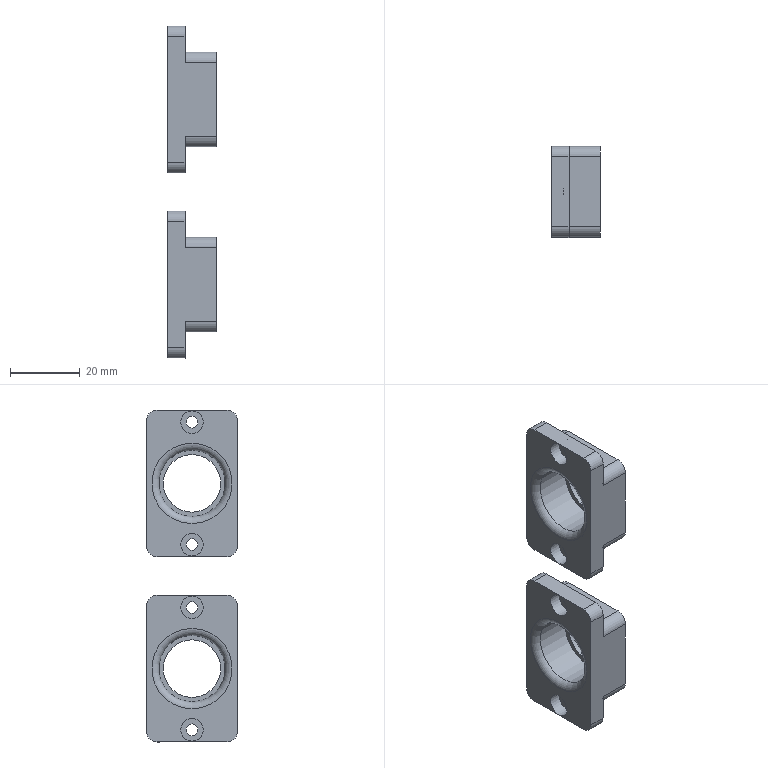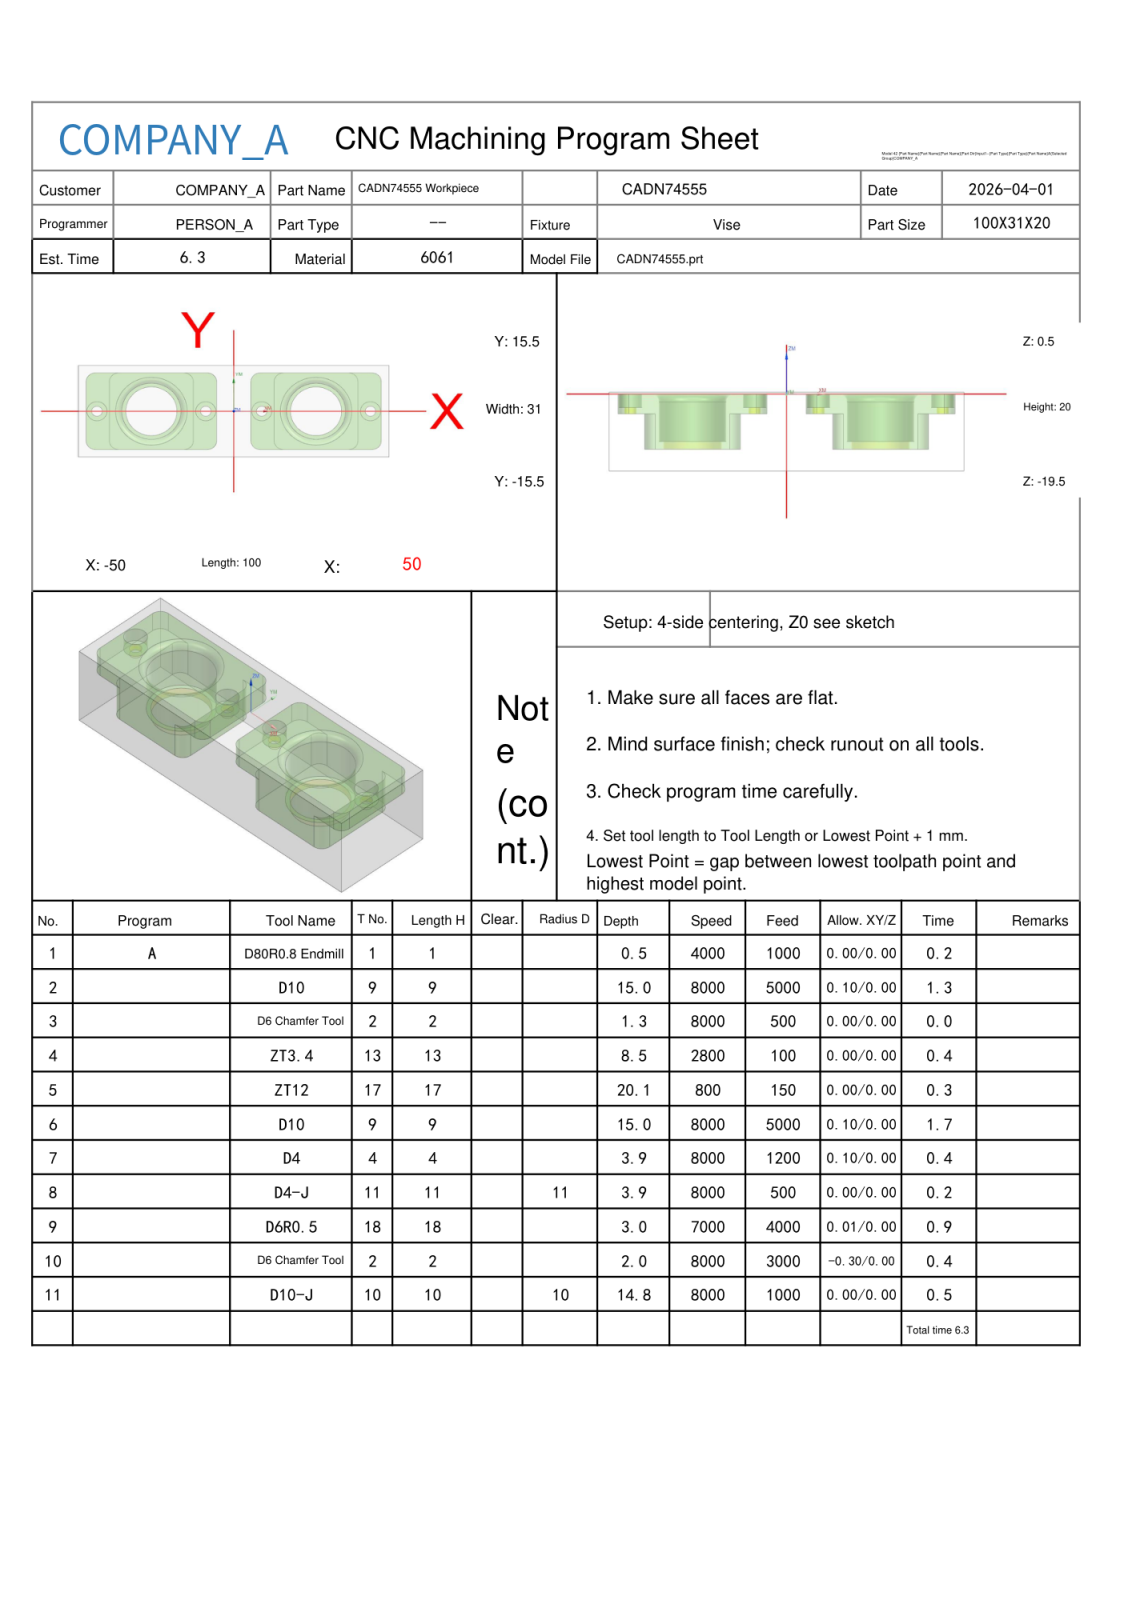NC program | NX | posted by the shop | part box 14 x 26 x 95 mm
Lines 427 to 1568 of 19918:
N6 T09 M06
(D10  D=10. R=0. H=09 ce=0.10 di=0.00)
G00 G90 G54 X-26.5 Y0.0 M03 S8000
G43 H09 Z20.
M08
Z.5
G03 X-28.7 Y-2.2 I0.0 J-2.2 F1200.
X-26.5 Y-4.4 I2.2 J0.0
X-26.5 Y-4.4 Z0.0 I0.0 J4.4
X-26.5 Y-4.4 Z-.5 I0.0 J4.4
X-26.5 Y-4.4 Z-1. I0.0 J4.4
X-26.5 Y-4.4 Z-1.5 I0.0 J4.4
X-26.5 Y-4.4 Z-2. I0.0 J4.4
X-26.5 Y-4.4 Z-2.5 I0.0 J4.4
X-26.5 Y-4.4 Z-3. I0.0 J4.4
X-26.5 Y-4.4 Z-3.5 I0.0 J4.4
X-26.5 Y-4.4 Z-4. I0.0 J4.4
X-26.5 Y-4.4 Z-4.5 I0.0 J4.4
X-26.5 Y-4.4 Z-5. I0.0 J4.4
X-26.5 Y-4.4 Z-5.5 I0.0 J4.4
X-26.5 Y-4.4 Z-6. I0.0 J4.4
X-26.5 Y-4.4 Z-6.5 I0.0 J4.4
X-26.5 Y-4.4 Z-7. I0.0 J4.4
X-26.5 Y-4.4 Z-7.5 I0.0 J4.4
X-26.5 Y-4.4 Z-8. I0.0 J4.4
X-26.5 Y-4.4 Z-8.5 I0.0 J4.4
X-26.5 Y-4.4 Z-9. I0.0 J4.4
X-26.5 Y-4.4 Z-9.5 I0.0 J4.4
X-26.5 Y-4.4 Z-10. I0.0 J4.4
X-26.5 Y-4.4 Z-10.5 I0.0 J4.4
X-26.5 Y-4.4 Z-11. I0.0 J4.4
X-26.5 Y-4.4 Z-11.5 I0.0 J4.4
X-26.5 Y-4.4 Z-12. I0.0 J4.4
X-22.1 Y0.0 I0.0 J4.4
X-26.5 Y4.4 I-4.4 J0.0
X-30.9 Y0.0 I0.0 J-4.4
X-26.5 Y-4.4 I4.4 J0.0
X-24.3 Y-2.2 I0.0 J2.2
X-26.5 Y0.0 I-2.2 J0.0
G00 Z20.
X26.5
Z.5
G03 X24.3 Y-2.2 I0.0 J-2.2
X26.5 Y-4.4 I2.2 J0.0
X26.5 Y-4.4 Z0.0 I0.0 J4.4
X26.5 Y-4.4 Z-.5 I0.0 J4.4
X26.5 Y-4.4 Z-1. I0.0 J4.4
X26.5 Y-4.4 Z-1.5 I0.0 J4.4
X26.5 Y-4.4 Z-2. I0.0 J4.4
X26.5 Y-4.4 Z-2.5 I0.0 J4.4
X26.5 Y-4.4 Z-3. I0.0 J4.4
X26.5 Y-4.4 Z-3.5 I0.0 J4.4
X26.5 Y-4.4 Z-4. I0.0 J4.4
X26.5 Y-4.4 Z-4.5 I0.0 J4.4
X26.5 Y-4.4 Z-5. I0.0 J4.4
X26.5 Y-4.4 Z-5.5 I0.0 J4.4
X26.5 Y-4.4 Z-6. I0.0 J4.4
X26.5 Y-4.4 Z-6.5 I0.0 J4.4
X26.5 Y-4.4 Z-7. I0.0 J4.4
X26.5 Y-4.4 Z-7.5 I0.0 J4.4
X26.5 Y-4.4 Z-8. I0.0 J4.4
X26.5 Y-4.4 Z-8.5 I0.0 J4.4
X26.5 Y-4.4 Z-9. I0.0 J4.4
X26.5 Y-4.4 Z-9.5 I0.0 J4.4
X26.5 Y-4.4 Z-10. I0.0 J4.4
X26.5 Y-4.4 Z-10.5 I0.0 J4.4
X26.5 Y-4.4 Z-11. I0.0 J4.4
X26.5 Y-4.4 Z-11.5 I0.0 J4.4
X26.5 Y-4.4 Z-12. I0.0 J4.4
X30.9 Y0.0 I0.0 J4.4
X26.5 Y4.4 I-4.4 J0.0
X22.1 Y0.0 I0.0 J-4.4
X26.5 Y-4.4 I4.4 J0.0
X28.7 Y-2.2 I0.0 J2.2
X26.5 Y0.0 I-2.2 J0.0
G00 Z20.
G00 G90 X-25.701 Y-3.038 M03 S8000
Z20.
Z-11.
G01 X-25.084 Y-2.847 Z-11.034 F2000.
X-24.251 Y-2.249 Z-11.088
X-23.653 Y-1.416 Z-11.141
X-23.35 Y-.436 Z-11.195
Y.436 Z-11.241
X-23.653 Y1.416 Z-11.295
X-24.251 Y2.249 Z-11.348
X-25.084 Y2.847 Z-11.402
X-26.064 Y3.15 Z-11.456
X-26.936 Z-11.501
X-27.916 Y2.847 Z-11.555
X-28.749 Y2.249 Z-11.609
X-29.347 Y1.416 Z-11.663
X-29.65 Y.436 Z-11.716
Y-.436 Z-11.762
X-29.347 Y-1.416 Z-11.816
X-28.749 Y-2.249 Z-11.87
X-27.916 Y-2.847 Z-11.923
X-26.936 Y-3.15 Z-11.977
X-26.5 Z-12.
G03 X-23.35 Y0.0 Z-12.069 I0.0 J3.15
X-26.5 Y3.15 Z-12.139 I-3.15 J0.0
X-29.65 Y0.0 Z-12.208 I0.0 J-3.15
X-26.5 Y-3.15 Z-12.278 I3.15 J0.0
X-23.35 Y0.0 Z-12.347 I0.0 J3.15
X-26.5 Y3.15 Z-12.417 I-3.15 J0.0
X-29.65 Y0.0 Z-12.486 I0.0 J-3.15
X-26.5 Y-3.15 Z-12.556 I3.15 J0.0
X-23.35 Y0.0 Z-12.625 I0.0 J3.15
X-26.5 Y3.15 Z-12.694 I-3.15 J0.0
X-29.65 Y0.0 Z-12.764 I0.0 J-3.15
X-26.5 Y-3.15 Z-12.833 I3.15 J0.0
X-23.35 Y0.0 Z-12.903 I0.0 J3.15
X-26.5 Y3.15 Z-12.972 I-3.15 J0.0
X-29.65 Y0.0 Z-13.042 I0.0 J-3.15
X-26.5 Y-3.15 Z-13.111 I3.15 J0.0
X-23.35 Y0.0 Z-13.181 I0.0 J3.15
X-26.5 Y3.15 Z-13.25 I-3.15 J0.0
X-29.65 Y0.0 Z-13.319 I0.0 J-3.15
X-26.5 Y-3.15 Z-13.389 I3.15 J0.0
X-23.35 Y0.0 Z-13.458 I0.0 J3.15
X-26.5 Y3.15 Z-13.528 I-3.15 J0.0
X-29.65 Y0.0 Z-13.597 I0.0 J-3.15
X-26.5 Y-3.15 Z-13.667 I3.15 J0.0
X-23.35 Y0.0 Z-13.736 I0.0 J3.15
X-26.5 Y3.15 Z-13.806 I-3.15 J0.0
X-29.65 Y0.0 Z-13.875 I0.0 J-3.15
X-26.5 Y-3.15 Z-13.944 I3.15 J0.0
X-23.35 Y0.0 Z-14.014 I0.0 J3.15
X-26.5 Y3.15 Z-14.083 I-3.15 J0.0
X-29.65 Y0.0 Z-14.153 I0.0 J-3.15
X-26.5 Y-3.15 Z-14.222 I3.15 J0.0
X-23.35 Y0.0 Z-14.292 I0.0 J3.15
X-26.5 Y3.15 Z-14.361 I-3.15 J0.0
X-29.65 Y0.0 Z-14.431 I0.0 J-3.15
X-26.5 Y-3.15 Z-14.5 I3.15 J0.0
X-23.35 Y0.0 I0.0 J3.15
X-26.5 Y3.15 I-3.15 J0.0
X-29.65 Y0.0 I0.0 J-3.15
X-26.5 Y-3.15 I3.15 J0.0
X-26.101 Y-3.125 I0.0 J3.15
G01 Z-13.5
G00 Z20.
X27.299 Y-3.038
Z-11.
G01 X27.916 Y-2.847 Z-11.034
X28.749 Y-2.249 Z-11.088
X29.347 Y-1.416 Z-11.141
X29.65 Y-.436 Z-11.195
Y.436 Z-11.241
X29.347 Y1.416 Z-11.295
X28.749 Y2.249 Z-11.348
X27.916 Y2.847 Z-11.402
X26.936 Y3.15 Z-11.456
X26.064 Z-11.501
X25.084 Y2.847 Z-11.555
X24.251 Y2.249 Z-11.609
X23.653 Y1.416 Z-11.663
X23.35 Y.436 Z-11.716
Y-.436 Z-11.762
X23.653 Y-1.416 Z-11.816
X24.251 Y-2.249 Z-11.87
X25.084 Y-2.847 Z-11.923
X26.064 Y-3.15 Z-11.977
X26.5 Z-12.
G03 X29.65 Y0.0 Z-12.069 I0.0 J3.15
X26.5 Y3.15 Z-12.139 I-3.15 J0.0
X23.35 Y0.0 Z-12.208 I0.0 J-3.15
X26.5 Y-3.15 Z-12.278 I3.15 J0.0
X29.65 Y0.0 Z-12.347 I0.0 J3.15
X26.5 Y3.15 Z-12.417 I-3.15 J0.0
X23.35 Y0.0 Z-12.486 I0.0 J-3.15
X26.5 Y-3.15 Z-12.556 I3.15 J0.0
X29.65 Y0.0 Z-12.625 I0.0 J3.15
X26.5 Y3.15 Z-12.694 I-3.15 J0.0
X23.35 Y0.0 Z-12.764 I0.0 J-3.15
X26.5 Y-3.15 Z-12.833 I3.15 J0.0
X29.65 Y0.0 Z-12.903 I0.0 J3.15
X26.5 Y3.15 Z-12.972 I-3.15 J0.0
X23.35 Y0.0 Z-13.042 I0.0 J-3.15
X26.5 Y-3.15 Z-13.111 I3.15 J0.0
X29.65 Y0.0 Z-13.181 I0.0 J3.15
X26.5 Y3.15 Z-13.25 I-3.15 J0.0
X23.35 Y0.0 Z-13.319 I0.0 J-3.15
X26.5 Y-3.15 Z-13.389 I3.15 J0.0
X29.65 Y0.0 Z-13.458 I0.0 J3.15
X26.5 Y3.15 Z-13.528 I-3.15 J0.0
X23.35 Y0.0 Z-13.597 I0.0 J-3.15
X26.5 Y-3.15 Z-13.667 I3.15 J0.0
X29.65 Y0.0 Z-13.736 I0.0 J3.15
X26.5 Y3.15 Z-13.806 I-3.15 J0.0
X23.35 Y0.0 Z-13.875 I0.0 J-3.15
X26.5 Y-3.15 Z-13.944 I3.15 J0.0
X29.65 Y0.0 Z-14.014 I0.0 J3.15
X26.5 Y3.15 Z-14.083 I-3.15 J0.0
X23.35 Y0.0 Z-14.153 I0.0 J-3.15
X26.5 Y-3.15 Z-14.222 I3.15 J0.0
X29.65 Y0.0 Z-14.292 I0.0 J3.15
X26.5 Y3.15 Z-14.361 I-3.15 J0.0
X23.35 Y0.0 Z-14.431 I0.0 J-3.15
X26.5 Y-3.15 Z-14.5 I3.15 J0.0
X29.65 Y0.0 I0.0 J3.15
X26.5 Y3.15 I-3.15 J0.0
X23.35 Y0.0 I0.0 J-3.15
X26.5 Y-3.15 I3.15 J0.0
X26.899 Y-3.125 I0.0 J3.15
G01 Z-13.5
G00 Z20.
G00 G90 X-20.384 Y-.188 M03 S7000
Z20.
Z1.5
G01 X-20.4 Y.489 Z1.464 F5000.
X-20.495 Y1.179 Z1.428
X-20.668 Y1.854 Z1.391
X-20.916 Y2.505 Z1.355
X-21.237 Y3.123 Z1.318
X-21.507 Y3.538 Z1.293
X-21.942 Y4.084 Z1.256
X-22.437 Y4.577 Z1.219
X-22.985 Y5.01 Z1.183
X-23.579 Y5.378 Z1.146
X-24.211 Y5.675 Z1.11
X-24.872 Y5.899 Z1.073
X-25.555 Y6.046 Z1.036
X-26.25 Y6.115 Z1.
X-26.949 Y6.103 Z.963
X-27.641 Y6.012 Z.927
X-28.319 Y5.843 Z.89
X-28.973 Y5.598 Z.853
X-29.594 Y5.28 Z.817
X-30.176 Y4.893 Z.78
X-30.709 Y4.442 Z.743
X-31.188 Y3.934 Z.707
X-31.606 Y3.374 Z.67
X-31.862 Y2.95 Z.644
X-32.151 Y2.348 Z.609
X-32.374 Y1.718 Z.574
X-32.526 Y1.067 Z.539
X-32.606 Y.403 Z.504
X-32.614 Y-.265 Z.469
X-32.549 Y-.93 Z.434
X-32.411 Y-1.584 Z.399
X-32.203 Y-2.22 Z.364
X-31.927 Y-2.828 Z.329
X-31.586 Y-3.403 Z.294
X-31.185 Y-3.938 Z.259
X-30.727 Y-4.425 Z.224
X-30.219 Y-4.86 Z.189
X-29.667 Y-5.236 Z.154
X-29.077 Y-5.551 Z.119
X-28.457 Y-5.799 Z.084
X-27.982 Y-5.938 Z.058
X-27.369 Y-6.058 Z.025
X-26.747 Y-6.115 Z-.007
X-26.5 Z-.02
G03 X-20.385 Y0.0 I0.0 J6.115
X-26.5 Y6.115 I-6.115 J0.0
X-32.615 Y0.0 I0.0 J-6.115
X-26.5 Y-6.115 I6.115 J0.0
G01 X-26.301 Y-6.11 Z-.021
X-26.103 Y-6.099
X-26.056 Y-6.095
X-26.008 Y-6.092
X-25.858 Y-6.076
X-25.708 Y-6.058
X-25.464 Y-6.019 Z-.022
X-25.223 Y-5.971
X-24.984 Y-5.913
X-24.747 Y-5.845
X-24.513 Y-5.768 Z-.023
X-24.283 Y-5.681
X-24.169 Y-5.635
X-24.056 Y-5.586
X-23.945 Y-5.535
X-23.834 Y-5.481
X-23.724 Y-5.426 Z-.024
X-23.616 Y-5.368
X-23.509 Y-5.308
X-23.403 Y-5.246
X-23.298 Y-5.181
X-23.194 Y-5.115
X-23.092 Y-5.047
X-22.992 Y-4.976
X-22.795 Y-4.83 Z-.025
X-22.604 Y-4.675
X-22.42 Y-4.513
X-22.242 Y-4.343
X-22.072 Y-4.167 Z-.026
X-21.909 Y-3.984
X-21.753 Y-3.795
X-21.605 Y-3.599 Z-.027
X-21.465 Y-3.398
X-21.334 Y-3.192
X-21.211 Y-2.98
X-21.096 Y-2.763 Z-.028
X-21.042 Y-2.654
X-20.991 Y-2.543
X-20.941 Y-2.431
X-20.894 Y-2.318
X-20.849 Y-2.204
X-20.806 Y-2.089
X-20.766 Y-1.974
X-20.728 Y-1.858 Z-.029
X-20.66 Y-1.623
X-20.6 Y-1.386
X-20.551 Y-1.146
X-20.511 Y-.905 Z-.03
X-20.481 Y-.663
X-20.46 Y-.42
X-20.45 Y-.176
X-20.449 Y.068 Z-.031
X-20.458 Y.312
X-20.477 Y.556
X-20.506 Y.798
X-20.544 Y1.039 Z-.032
X-20.592 Y1.278
X-20.65 Y1.514
X-20.683 Y1.632
X-20.717 Y1.749
X-20.754 Y1.865 Z-.033
X-20.794 Y1.98
X-20.836 Y2.094
X-20.88 Y2.208
X-20.926 Y2.32
X-20.975 Y2.432
X-21.078 Y2.652 Z-.034
X-21.191 Y2.868
X-21.249 Y2.972
X-21.31 Y3.075
X-21.375 Y3.181
X-21.442 Y3.285
X-21.58 Y3.486 Z-.035
X-21.726 Y3.681
X-21.88 Y3.871
X-22.041 Y4.053
X-22.209 Y4.229 Z-.036
X-22.385 Y4.398
X-22.567 Y4.56
X-22.755 Y4.714
X-22.95 Y4.861 Z-.037
X-23.15 Y4.999
X-23.355 Y5.129
X-23.566 Y5.251
X-23.673 Y5.309 Z-.038
X-23.781 Y5.364
X-23.891 Y5.418
X-24.001 Y5.469
X-24.112 Y5.518
X-24.225 Y5.564
X-24.338 Y5.608
X-24.452 Y5.65
X-24.683 Y5.727 Z-.039
X-24.916 Y5.795
X-25.152 Y5.853
X-25.39 Y5.901
X-25.629 Y5.94 Z-.04
X-25.871 Y5.969
X-26.112 Y5.989
X-26.355 Y5.998
X-26.597 Z-.041
X-26.84 Y5.988
X-27.082 Y5.968
X-27.322 Y5.938 Z-.042
X-27.561 Y5.899
X-27.799 Y5.85
X-28.034 Y5.791
X-28.266 Y5.723 Z-.043
X-28.382 Y5.686
X-28.496 Y5.646
X-28.609 Y5.604
X-28.722 Y5.56
X-28.834 Y5.513
X-28.945 Y5.464
X-29.054 Y5.413
X-29.163 Y5.36 Z-.044
X-29.377 Y5.247
X-29.586 Y5.125
X-29.79 Y4.995
X-29.989 Y4.857 Z-.045
X-30.182 Y4.711
X-30.368 Y4.557
X-30.548 Y4.397
X-30.722 Y4.228 Z-.046
X-30.889 Y4.053
X-31.048 Y3.872
X-31.2 Y3.684
X-31.344 Y3.49 Z-.047
X-31.405 Y3.403
X-31.465 Y3.315
X-31.538 Y3.201
X-31.608 Y3.086
X-31.726 Y2.88
X-31.835 Y2.67 Z-.048
X-31.936 Y2.455
X-32.029 Y2.237
X-32.112 Y2.015
X-32.187 Y1.789 Z-.049
X-32.252 Y1.562
X-32.309 Y1.332
X-32.356 Y1.099
X-32.394 Y.866 Z-.05
X-32.423 Y.63
X-32.442 Y.394
X-32.452 Y.158
Y-.079 Z-.051
X-32.443 Y-.315
X-32.425 Y-.551
X-32.397 Y-.786
X-32.36 Y-1.02 Z-.052
X-32.314 Y-1.252
X-32.259 Y-1.482
X-32.194 Y-1.709
X-32.121 Y-1.934 Z-.053
X-32.038 Y-2.155
X-31.947 Y-2.374
X-31.848 Y-2.588
X-31.74 Y-2.798 Z-.054
X-31.623 Y-3.003
X-31.499 Y-3.204
X-31.367 Y-3.4
X-31.227 Y-3.59 Z-.055
X-31.08 Y-3.774
X-30.925 Y-3.953
X-30.764 Y-4.125
X-30.596 Y-4.29 Z-.056
X-30.421 Y-4.449
X-30.241 Y-4.601
X-30.054 Y-4.745
X-29.862 Y-4.881 Z-.057
X-29.665 Y-5.01
X-29.463 Y-5.131
X-29.256 Y-5.244
X-29.045 Y-5.349 Z-.058
X-28.83 Y-5.445
X-28.611 Y-5.532
X-28.574 Y-5.546
X-28.537 Y-5.559
X-28.352 Y-5.623
X-28.164 Y-5.68 Z-.059
X-27.961 Y-5.735
X-27.755 Y-5.783
X-27.548 Y-5.823
X-27.34 Y-5.856 Z-.06
X-27.131 Y-5.881
X-26.921 Y-5.899
X-26.711 Y-5.909
X-26.5 Y-5.912
X-26.262 Y-5.906 Z-.061
X-26.024 Y-5.89
X-25.852 Y-5.872 Z-.062
X-25.681 Y-5.85
X-25.615 Y-5.84
X-25.55 Y-5.829
X-25.315 Y-5.784
X-25.082 Y-5.73 Z-.063
X-24.852 Y-5.666
X-24.624 Y-5.594 Z-.064
X-24.4 Y-5.512
X-24.179 Y-5.421
X-23.962 Y-5.321 Z-.065
X-23.749 Y-5.212
X-23.541 Y-5.096 Z-.066
X-23.338 Y-4.97
X-23.14 Y-4.837
X-22.948 Y-4.696 Z-.067
X-22.762 Y-4.547
X-22.582 Y-4.391
X-22.408 Y-4.228 Z-.068
X-22.241 Y-4.057
X-22.082 Y-3.881 Z-.069
X-21.929 Y-3.698
X-21.784 Y-3.509
X-21.647 Y-3.314 Z-.07
X-21.518 Y-3.114
X-21.398 Y-2.909 Z-.071
X-21.285 Y-2.7
X-21.182 Y-2.486
X-21.087 Y-2.268 Z-.072
X-21.001 Y-2.046
X-20.923 Y-1.821 Z-.073
X-20.856 Y-1.594
X-20.797 Y-1.364
X-20.748 Y-1.131 Z-.074
X-20.708 Y-.897
X-20.678 Y-.662
X-20.657 Y-.425 Z-.075
X-20.646 Y-.188
X-20.645 Y.049 Z-.076
X-20.653 Y.286
X-20.671 Y.522
X-20.698 Y.758 Z-.077
X-20.735 Y.992
X-20.781 Y1.224 Z-.078
X-20.836 Y1.454
X-20.901 Y1.682
X-20.975 Y1.907 Z-.079
X-21.058 Y2.128
X-21.15 Y2.347
X-21.251 Y2.561 Z-.08
X-21.36 Y2.77
X-21.477 Y2.976 Z-.081
X-21.508 Y3.026
X-21.539 Y3.076
X-21.635 Y3.224
X-21.736 Y3.37
X-21.877 Y3.558 Z-.082
X-22.025 Y3.741
X-22.18 Y3.918 Z-.083
X-22.343 Y4.088
X-22.512 Y4.251
X-22.688 Y4.408 Z-.084
X-22.87 Y4.557
X-23.057 Y4.699
X-23.25 Y4.833 Z-.085
X-23.449 Y4.959
X-23.652 Y5.077 Z-.086
X-23.859 Y5.187
X-24.071 Y5.288
X-24.287 Y5.38 Z-.087
X-24.507 Y5.464
X-24.729 Y5.539 Z-.088
X-24.954 Y5.605
X-25.182 Y5.661
X-25.412 Y5.708 Z-.089
X-25.643 Y5.746
X-25.876 Y5.775
X-26.109 Y5.794 Z-.09
X-26.343 Y5.804
X-26.578 Y5.805 Z-.091
X-26.812 Y5.796
X-27.045 Y5.777
X-27.278 Y5.749 Z-.092
X-27.509 Y5.712
X-27.738 Y5.665
X-27.966 Y5.61 Z-.093
X-28.19 Y5.545
X-28.412 Y5.471 Z-.094
X-28.631 Y5.388
X-28.846 Y5.297
X-29.058 Y5.197 Z-.095
X-29.265 Y5.088
X-29.467 Y4.971 Z-.096
X-29.665 Y4.847
X-29.857 Y4.714
X-30.044 Y4.574 Z-.097
X-30.224 Y4.426
X-30.399 Y4.271
X-30.568 Y4.11 Z-.098
X-30.729 Y3.942
X-30.884 Y3.767 Z-.099
X-31.032 Y3.586
X-31.172 Y3.4
X-31.304 Y3.208 Z-.1
X-31.357 Y3.126
X-31.409 Y3.044
X-31.48 Y2.923
X-31.549 Y2.801
X-31.659 Y2.591 Z-.101
X-31.76 Y2.377
X-31.852 Y2.158 Z-.102
X-31.935 Y1.936
X-32.009 Y1.711
X-32.073 Y1.482 Z-.103
X-32.129 Y1.252
X-32.174 Y1.019 Z-.104
X-32.21 Y.785
X-32.236 Y.55
X-32.253 Y.314 Z-.105
X-32.26 Y.077
X-32.257 Y-.16
X-32.244 Y-.396 Z-.106
X-32.222 Y-.631
X-32.19 Y-.866 Z-.107
X-32.149 Y-1.099
X-32.098 Y-1.33
X-32.037 Y-1.558 Z-.108
X-31.968 Y-1.784
X-31.889 Y-2.007 Z-.109
X-31.801 Y-2.226
X-31.704 Y-2.441
X-31.598 Y-2.653 Z-.11
X-31.484 Y-2.859
X-31.361 Y-3.061
X-31.23 Y-3.258 Z-.111
X-31.092 Y-3.449
X-30.945 Y-3.634 Z-.112
X-30.791 Y-3.812
X-30.63 Y-3.985
X-30.462 Y-4.15 Z-.113
X-30.288 Y-4.309
X-30.107 Y-4.46 Z-.114
X-29.92 Y-4.603
X-29.727 Y-4.739
X-29.529 Y-4.867 Z-.115
X-29.326 Y-4.986
X-29.118 Y-5.097
X-28.906 Y-5.2 Z-.116
X-28.69 Y-5.293
X-28.471 Y-5.378 Z-.117
X-28.28 Y-5.442
X-28.088 Y-5.501
X-27.981 Y-5.53
X-27.874 Y-5.557 Z-.118
X-27.786 Y-5.578
X-27.697 Y-5.597
X-27.5 Y-5.635
X-27.301 Y-5.665 Z-.119
X-27.102 Y-5.689
X-26.901 Y-5.706
X-26.701 Y-5.715 Z-.12
X-26.5 Y-5.718
X-26.301 Y-5.713
X-26.103 Y-5.702 Z-.121
X-25.905 Y-5.683
X-25.681 Y-5.654 Z-.122
X-25.461 Y-5.617
X-25.243 Y-5.57 Z-.123
X-25.014 Y-5.512
X-24.788 Y-5.445 Z-.124
X-24.564 Y-5.368
X-24.344 Y-5.282 Z-.125
X-24.128 Y-5.187
X-23.916 Y-5.083 Z-.126
X-23.709 Y-4.971
X-23.506 Y-4.85 Z-.127
X-23.309 Y-4.72
X-23.117 Y-4.583 Z-.128
X-22.931 Y-4.438
X-22.752 Y-4.286 Z-.129
X-22.579 Y-4.126
X-22.412 Y-3.959 Z-.13
X-22.253 Y-3.786 Z-.131
X-22.101 Y-3.606
X-21.957 Y-3.42 Z-.132
X-21.82 Y-3.228
X-21.692 Y-3.031 Z-.133
X-21.572 Y-2.829
X-21.46 Y-2.622 Z-.134
X-21.357 Y-2.411
X-21.263 Y-2.195 Z-.135
X-21.178 Y-1.976
X-21.102 Y-1.754 Z-.136
X-21.035 Y-1.529
X-20.978 Y-1.301 Z-.137
X-20.93 Y-1.071
X-20.892 Y-.839 Z-.138
X-20.863 Y-.606
X-20.844 Y-.373 Z-.139
X-20.835 Y-.138
X-20.836 Y.096 Z-.14
X-20.846 Y.33
X-20.865 Y.564 Z-.141
X-20.895 Y.797
X-20.934 Y1.027 Z-.142
X-20.983 Y1.257
X-21.04 Y1.483 Z-.143
X-21.108 Y1.708 Z-.144
X-21.184 Y1.929
X-21.27 Y2.147 Z-.145
X-21.364 Y2.361
X-21.468 Y2.571 Z-.146
X-21.579 Y2.776
X-21.7 Y2.977 Z-.147
X-21.731 Y3.027
X-21.764 Y3.076
X-21.859 Y3.217
X-21.959 Y3.355 Z-.148
X-22.1 Y3.536
X-22.248 Y3.711 Z-.149
X-22.403 Y3.88
X-22.565 Y4.042 Z-.15
X-22.733 Y4.198
X-22.908 Y4.346 Z-.151
X-23.088 Y4.487
X-23.274 Y4.621 Z-.152
X-23.465 Y4.748
X-23.661 Y4.866 Z-.153
X-23.861 Y4.976
X-24.066 Y5.078 Z-.154
X-24.275 Y5.172
X-24.487 Y5.257 Z-.155
X-24.703 Y5.333
X-24.921 Y5.4 Z-.156
X-25.142 Y5.459
X-25.365 Y5.508 Z-.157
X-25.59 Y5.549
X-25.816 Y5.58 Z-.158
X-26.044 Y5.602
X-26.272 Y5.615 Z-.159
X-26.5 Y5.618
X-26.728 Y5.612 Z-.16
X-26.956 Y5.597
X-27.183 Y5.573 Z-.161
X-27.408 Y5.539
X-27.632 Y5.497 Z-.162
X-27.854 Y5.445
X-28.074 Y5.384 Z-.163
X-28.291 Y5.315
X-28.505 Y5.237 Z-.164
X-28.716 Y5.15
X-28.922 Y5.054 Z-.165
X-29.125 Y4.951
X-29.324 Y4.839 Z-.166
X-29.517 Y4.72
X-29.706 Y4.592 Z-.167
X-29.889 Y4.457
X-30.066 Y4.315 Z-.168
X-30.238 Y4.166
X-30.403 Y4.01 Z-.169
X-30.562 Y3.847
X-30.714 Y3.678 Z-.17
X-30.859 Y3.503
X-30.997 Y3.323 Z-.171
X-31.094 Y3.185
X-31.188 Y3.045 Z-.172
X-31.219 Y2.995
X-31.25 Y2.945
X-31.365 Y2.748
X-31.473 Y2.546 Z-.173
X-31.572 Y2.34
X-31.662 Y2.13 Z-.174
X-31.744 Y1.916
X-31.817 Y1.7 Z-.175
X-31.881 Y1.48
X-31.936 Y1.258 Z-.176
X-31.982 Y1.035
X-32.019 Y.809 Z-.177
X-32.046 Y.583
X-32.064 Y.355 Z-.178
X-32.073 Y.127
X-32.072 Y-.101 Z-.179
X-32.062 Y-.329
X-32.043 Y-.557 Z-.18
X-32.015 Y-.783
X-31.977 Y-1.008 Z-.181
X-31.93 Y-1.231
X-31.874 Y-1.452 Z-.182
X-31.809 Y-1.67
X-31.735 Y-1.886 Z-.183
X-31.652 Y-2.098 Z-.184
X-31.561 Y-2.307
X-31.462 Y-2.511 Z-.185
X-31.354 Y-2.712
X-31.238 Y-2.908 Z-.186
X-31.114 Y-3.099
X-30.982 Y-3.284 Z-.187
X-30.843 Y-3.464
X-30.697 Y-3.639 Z-.188
X-30.544 Y-3.807
X-30.384 Y-3.968 Z-.189
X-30.217 Y-4.123
X-30.045 Y-4.271 Z-.19
X-29.866 Y-4.411
X-29.682 Y-4.545 Z-.191
X-29.493 Y-4.67
X-29.299 Y-4.788 Z-.192
X-29.1 Y-4.898
X-28.897 Y-4.999 Z-.193
X-28.69 Y-5.092
X-28.494 Y-5.171 Z-.194
X-28.296 Y-5.242
X-28.281 Y-5.247
X-28.265 Y-5.252
X-28.048 Y-5.319 Z-.195
X-27.829 Y-5.377
X-27.611 Y-5.425 Z-.196
X-27.391 Y-5.464
X-27.169 Y-5.495 Z-.197
X-26.947 Y-5.516
X-26.723 Y-5.529 Z-.198
X-26.5 Y-5.532
X-26.301 Y-5.528 Z-.199
X-26.103 Y-5.516
X-26.056 Y-5.512
X-26.009 Y-5.508
X-25.858 Y-5.491 Z-.2
X-25.708 Y-5.471
X-25.48 Y-5.432 Z-.201
X-25.255 Y-5.383 Z-.202
X-25.032 Y-5.325
X-24.811 Y-5.258 Z-.203
X-24.594 Y-5.182 Z-.204
X-24.38 Y-5.096
X-24.17 Y-5.002 Z-.205
X-23.964 Y-4.9
X-23.762 Y-4.788 Z-.206
X-23.566 Y-4.669 Z-.207
X-23.374 Y-4.541
X-23.188 Y-4.406 Z-.208
X-23.008 Y-4.263 Z-.209
X-22.834 Y-4.113
X-22.667 Y-3.955 Z-.21
X-22.506 Y-3.791 Z-.211
X-22.352 Y-3.62
X-22.206 Y-3.443 Z-.212
X-22.067 Y-3.26 Z-.213
X-21.936 Y-3.072
X-21.813 Y-2.878 Z-.214
X-21.698 Y-2.679 Z-.215
X-21.592 Y-2.476
X-21.494 Y-2.269 Z-.216
X-21.405 Y-2.057
X-21.324 Y-1.843 Z-.217
X-21.253 Y-1.625 Z-.218
X-21.191 Y-1.404
X-21.138 Y-1.181 Z-.219
X-21.095 Y-.956 Z-.22
X-21.061 Y-.73
X-21.037 Y-.502 Z-.221
X-21.022 Y-.274 Z-.222
X-21.016 Y-.045
X-21.021 Y.184 Z-.223
X-21.034 Y.412 Z-.224
X-21.057 Y.64
X-21.09 Y.866 Z-.225
X-21.132 Y1.091
X-21.183 Y1.313 Z-.226
X-21.244 Y1.534 Z-.227
X-21.314 Y1.751
X-21.392 Y1.966 Z-.228
X-21.48 Y2.176 Z-.229
X-21.576 Y2.383
X-21.681 Y2.586 Z-.23
X-21.728 Y2.67
X-21.775 Y2.753
X-21.844 Y2.866 Z-.231
X-21.916 Y2.978
X-22.044 Y3.164 Z-.232
X-22.18 Y3.345 Z-.233
X-22.323 Y3.521
X-22.473 Y3.69 Z-.234
X-22.631 Y3.853
X-22.794 Y4.009 Z-.235
X-22.964 Y4.158 Z-.236
X-23.14 Y4.3
X-23.322 Y4.435 Z-.237
X-23.509 Y4.562 Z-.238
X-23.702 Y4.681
X-23.899 Y4.792 Z-.239
X-24.1 Y4.894 Z-.24
X-24.305 Y4.988
X-24.514 Y5.074 Z-.241
X-24.727 Y5.151
X-24.942 Y5.219 Z-.242
X-25.16 Y5.278 Z-.243
X-25.38 Y5.328
X-25.602 Y5.368 Z-.244
X-25.825 Y5.4 Z-.245
X-26.05 Y5.422
X-26.275 Y5.435 Z-.246
X-26.5 Y5.438
X-26.725 Y5.432 Z-.247
X-26.95 Y5.417 Z-.248
X-27.174 Y5.393
X-27.397 Y5.359 Z-.249
X-27.618 Y5.316 Z-.25
X-27.837 Y5.264
X-28.053 Y5.203 Z-.251
X-28.267 Y5.133 Z-.252
X-28.478 Y5.055
X-28.686 Y4.967 Z-.253
X-28.889 Y4.871
X-29.088 Y4.767 Z-.254
X-29.283 Y4.655 Z-.255
X-29.473 Y4.535
X-29.657 Y4.407 Z-.256
X-29.837 Y4.271 Z-.257
X-30.01 Y4.128
X-30.177 Y3.978 Z-.258
X-30.338 Y3.822 Z-.259
X-30.493 Y3.659
X-30.64 Y3.49 Z-.26
X-30.78 Y3.314
X-30.879 Y3.181 Z-.261
X-30.974 Y3.045
X-31.006 Y2.996 Z-.262
X-31.038 Y2.947
X-31.155 Y2.757
X-31.264 Y2.562 Z-.263
X-31.364 Y2.363 Z-.264
X-31.457 Y2.159
X-31.541 Y1.953 Z-.265
X-31.616 Y1.742
X-31.682 Y1.53 Z-.266
X-31.74 Y1.314 Z-.267
X-31.789 Y1.096
X-31.828 Y.877 Z-.268
X-31.859 Y.656 Z-.269
X-31.88 Y.434
X-31.893 Y.212 Z-.27
X-31.896 Y-.011
X-31.89 Y-.234 Z-.271
X-31.874 Y-.456 Z-.272
X-31.85 Y-.677
X-31.816 Y-.897 Z-.273
X-31.774 Y-1.116 Z-.274
X-31.722 Y-1.332
X-31.662 Y-1.546 Z-.275
X-31.592 Y-1.758
X-31.514 Y-1.966 Z-.276
X-31.428 Y-2.171 Z-.277
X-31.333 Y-2.372
X-31.23 Y-2.569 Z-.278
X-31.119 Y-2.762 Z-.279
X-31.001 Y-2.949
X-30.874 Y-3.132 Z-.28
X-30.74 Y-3.309
X-30.599 Y-3.481 Z-.281
X-30.451 Y-3.646 Z-.282
X-30.297 Y-3.805
X-30.136 Y-3.958 Z-.283
X-29.969 Y-4.104 Z-.284
X-29.795 Y-4.243
X-29.617 Y-4.375 Z-.285
X-29.433 Y-4.499
X-29.244 Y-4.615 Z-.286
X-29.051 Y-4.723 Z-.287
X-28.854 Y-4.824
X-28.652 Y-4.916 Z-.288
X-28.447 Y-4.999 Z-.289
X-28.238 Y-5.075
X-28.027 Y-5.141 Z-.29
X-27.814 Y-5.199
X-27.726 Y-5.219 Z-.291
X-27.639 Y-5.239
X-27.51 Y-5.265
X-27.381 Y-5.287 Z-.292
X-27.162 Y-5.318
X-26.942 Y-5.34 Z-.293
X-26.721 Y-5.352 Z-.294
X-26.5 Y-5.356
X-26.381 Y-5.354 Z-.295
X-26.262 Y-5.349
X-26.143 Y-5.342
X-26.009 Y-5.331 Z-.296
X-25.794 Y-5.305 Z-.297
X-25.581 Y-5.271
X-25.361 Y-5.227 Z-.298
X-25.144 Y-5.173 Z-.299
X-24.929 Y-5.111 Z-.3
X-24.717 Y-5.04
X-24.508 Y-4.959 Z-.301
X-24.302 Y-4.871 Z-.302
X-24.101 Y-4.773 Z-.303
X-23.904 Y-4.668
X-23.712 Y-4.554 Z-.304
X-23.524 Y-4.432 Z-.305
X-23.342 Y-4.303 Z-.306
X-23.165 Y-4.166
X-22.995 Y-4.022 Z-.307
X-22.83 Y-3.871 Z-.308
X-22.673 Y-3.713 Z-.309
X-22.521 Y-3.549 Z-.31
X-22.377 Y-3.378
X-22.24 Y-3.202 Z-.311
X-22.111 Y-3.02 Z-.312
X-21.99 Y-2.833 Z-.313
X-21.876 Y-2.642
X-21.771 Y-2.445 Z-.314
X-21.674 Y-2.245 Z-.315
X-21.585 Y-2.04 Z-.316
X-21.505 Y-1.832
X-21.434 Y-1.621 Z-.317
X-21.372 Y-1.408 Z-.318
X-21.318 Y-1.191 Z-.319
X-21.274 Y-.973
X-21.239 Y-.754 Z-.32
X-21.213 Y-.533 Z-.321
X-21.197 Y-.311 Z-.322
X-21.19 Y-.089
X-21.192 Y.134 Z-.323
X-21.203 Y.356 Z-.324
X-21.224 Y.577 Z-.325
X-21.254 Y.797 Z-.326
X-21.293 Y1.016
X-21.341 Y1.232 Z-.327
X-21.398 Y1.447 Z-.328
X-21.464 Y1.659 Z-.329
X-21.539 Y1.868
X-21.623 Y2.073 Z-.33
X-21.715 Y2.275 Z-.331
X-21.815 Y2.473 Z-.332
X-21.924 Y2.666
X-21.949 Y2.708 Z-.333
X-21.975 Y2.751
X-22.068 Y2.897
X-22.166 Y3.039 Z-.334
X-22.298 Y3.218 Z-.335
X-22.438 Y3.391
X-22.585 Y3.558 Z-.336
X-22.738 Y3.718 Z-.337
X-22.899 Y3.872 Z-.338
X-23.065 Y4.019
X-23.238 Y4.159 Z-.339
X-23.416 Y4.291 Z-.34
X-23.599 Y4.416 Z-.341
X-23.788 Y4.533
X-23.981 Y4.642 Z-.342
X-24.179 Y4.743 Z-.343
X-24.381 Y4.835 Z-.344
X-24.586 Y4.919
X-24.795 Y4.994 Z-.345
X-25.006 Y5.06 Z-.346
X-25.22 Y5.117 Z-.347
X-25.437 Y5.165 Z-.348
X-25.655 Y5.204
X-25.874 Y5.234 Z-.349
X-26.094 Y5.254 Z-.35
X-26.316 Y5.266 Z-.351
X-26.537 Y5.268
X-26.758 Y5.26 Z-.352
X-26.979 Y5.244 Z-.353
X-27.198 Y5.218 Z-.354
X-27.417 Y5.183
X-27.633 Y5.139 Z-.355
X-27.848 Y5.086 Z-.356
X-28.06 Y5.024 Z-.357
X-28.269 Y4.953
X-28.475 Y4.873 Z-.358
X-28.678 Y4.785 Z-.359
X-28.876 Y4.688 Z-.36
X-29.07 Y4.583
X-29.26 Y4.47 Z-.361
X-29.445 Y4.35 Z-.362
X-29.624 Y4.221 Z-.363
X-29.798 Y4.085
X-29.966 Y3.942 Z-.364
X-30.128 Y3.793 Z-.365
X-30.283 Y3.636 Z-.366
X-30.432 Y3.473
X-30.573 Y3.305 Z-.367
X-30.703 Y3.136 Z-.368
X-30.834 Y2.95 Z-.369
X-30.955 Y2.763
X-31.067 Y2.57 Z-.37
X-31.171 Y2.374 Z-.371
X-31.267 Y2.173 Z-.372
X-31.354 Y1.968
X-31.432 Y1.759 Z-.373
X-31.501 Y1.548 Z-.374
X-31.562 Y1.334 Z-.375
X-31.613 Y1.118 Z-.376
X-31.655 Y.899
X-31.687 Y.679 Z-.377
X-31.71 Y.458 Z-.378
X-31.724 Y.237 Z-.379
X-31.728 Y.014
X-31.723 Y-.208 Z-.38
X-31.708 Y-.429 Z-.381
X-31.684 Y-.65 Z-.382
X-31.651 Y-.869
X-31.609 Y-1.087 Z-.383
X-31.557 Y-1.303 Z-.384
X-31.496 Y-1.516 Z-.385
X-31.426 Y-1.727
X-31.347 Y-1.934 Z-.386
X-31.26 Y-2.138 Z-.387
X-31.164 Y-2.337 Z-.388
X-31.059 Y-2.533
X-30.947 Y-2.724 Z-.389
X-30.826 Y-2.909 Z-.39
X-30.698 Y-3.09 Z-.391
X-30.562 Y-3.265
X-30.419 Y-3.434 Z-.392
X-30.269 Y-3.596 Z-.393
X-30.112 Y-3.752 Z-.394
X-29.949 Y-3.902
X-29.779 Y-4.044 Z-.395
X-29.604 Y-4.179 Z-.396
X-29.423 Y-4.306 Z-.397
X-29.237 Y-4.425
X-29.046 Y-4.537 Z-.398
X-28.851 Y-4.64 Z-.399
X-28.651 Y-4.735 Z-.4
X-28.448 Y-4.821 Z-.401
X-28.308 Y-4.874
X-28.166 Y-4.924 Z-.402
X-28.099 Y-4.946
X-28.031 Y-4.967
X-27.818 Y-5.026 Z-.403
X-27.604 Y-5.077 Z-.404
X-27.422 Y-5.112
X-27.239 Y-5.141 Z-.405
X-27.055 Y-5.163
X-26.87 Y-5.179 Z-.406
X-26.685 Y-5.188 Z-.407
X-26.5 Y-5.19
X-26.381 Y-5.188 Z-.408
X-26.262 Y-5.184
X-26.143 Y-5.176 Z-.409
X-26.024 Y-5.166
X-25.854 Y-5.147 Z-.41
X-25.684 Y-5.122 Z-.411
X-25.637 Y-5.113
X-25.591 Y-5.106
X-25.377 Y-5.061 Z-.412
X-25.165 Y-5.009 Z-.413
X-24.955 Y-4.946 Z-.414
X-24.748 Y-4.876 Z-.415
X-24.544 Y-4.797
X-24.344 Y-4.709 Z-.416
X-24.148 Y-4.613 Z-.417
X-23.956 Y-4.508 Z-.418
X-23.769 Y-4.396 Z-.419
X-23.586 Y-4.276 Z-.42
X-23.41 Y-4.148 Z-.421
X-23.238 Y-4.014 Z-.422
X-23.072 Y-3.871
X-22.913 Y-3.723 Z-.423
X-22.76 Y-3.567 Z-.424
X-22.614 Y-3.406 Z-.425
X-22.474 Y-3.238 Z-.426
X-22.342 Y-3.065 Z-.427
X-22.218 Y-2.886 Z-.428
X-22.101 Y-2.702 Z-.429
X-21.991 Y-2.514
X-21.89 Y-2.321 Z-.43
X-21.798 Y-2.124 Z-.431
X-21.713 Y-1.923 Z-.432
X-21.638 Y-1.719 Z-.433
X-21.57 Y-1.512 Z-.434
X-21.512 Y-1.303 Z-.435
X-21.462 Y-1.091 Z-.436
X-21.422 Y-.877
X-21.391 Y-.662 Z-.437
X-21.369 Y-.446 Z-.438
X-21.355 Y-.229 Z-.439
X-21.351 Y-.012 Z-.44
X-21.356 Y.205 Z-.441
X-21.371 Y.422 Z-.442
X-21.394 Y.638 Z-.443
X-21.427 Y.852
X-21.468 Y1.066 Z-.444
X-21.519 Y1.276 Z-.445
X-21.578 Y1.485 Z-.446
X-21.646 Y1.691 Z-.447
X-21.723 Y1.894 Z-.448
X-21.808 Y2.093 Z-.449
X-21.901 Y2.289
X-22.003 Y2.48 Z-.45
X-22.112 Y2.667 Z-.451
X-22.138 Y2.708
X-22.163 Y2.748 Z-.452